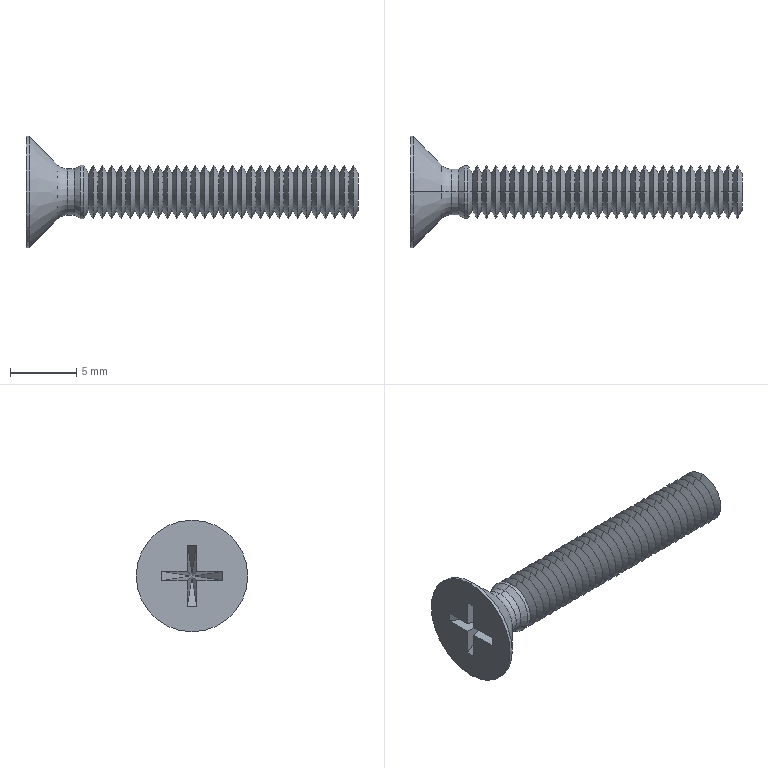Part | SolidWorks | features BlendCut 1, CirPattern 1, LPattern 1, RevCut 1, Revolution 1 | 1 solid | 144 faces | box 25 x 8.4 x 8.4 mm | volume 285.936 mm3 | cone 122 | plane 14 | cylinder 6 | torus 2 | commonest cylinder face diameters 3.464 x2 4 x2 8.4 x2